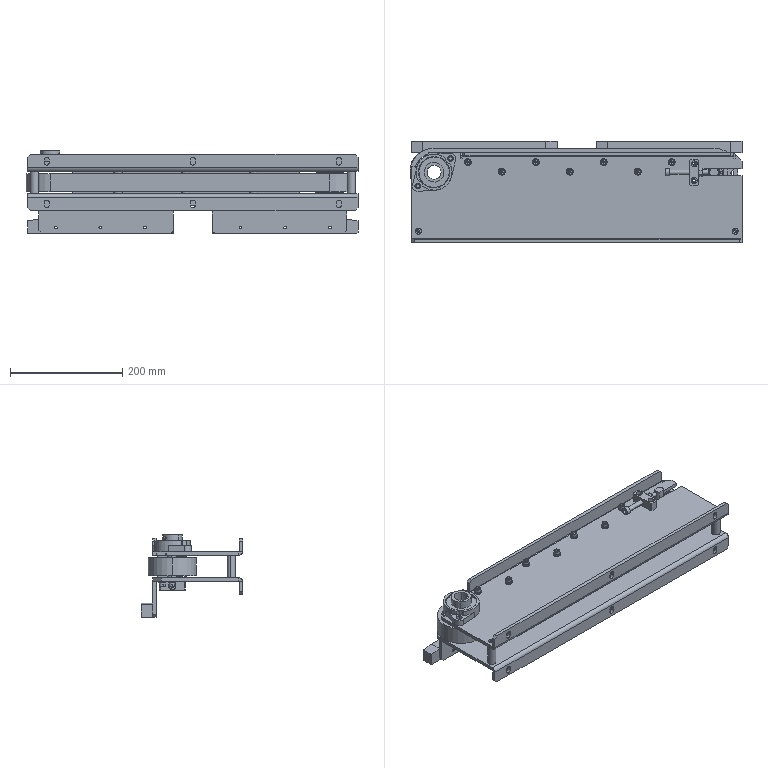Part | SolidWorks | 65 solids | 2073 faces | box 590.86 x 180 x 146.5 mm | volume 2644810 mm3 | cylinder 842 | plane 589 | spline 412 | cone 230 | commonest cylinder face diameters 30.636 x144 8.51 x92 12 x70 76.481 x68 10 x56 6.1 x42